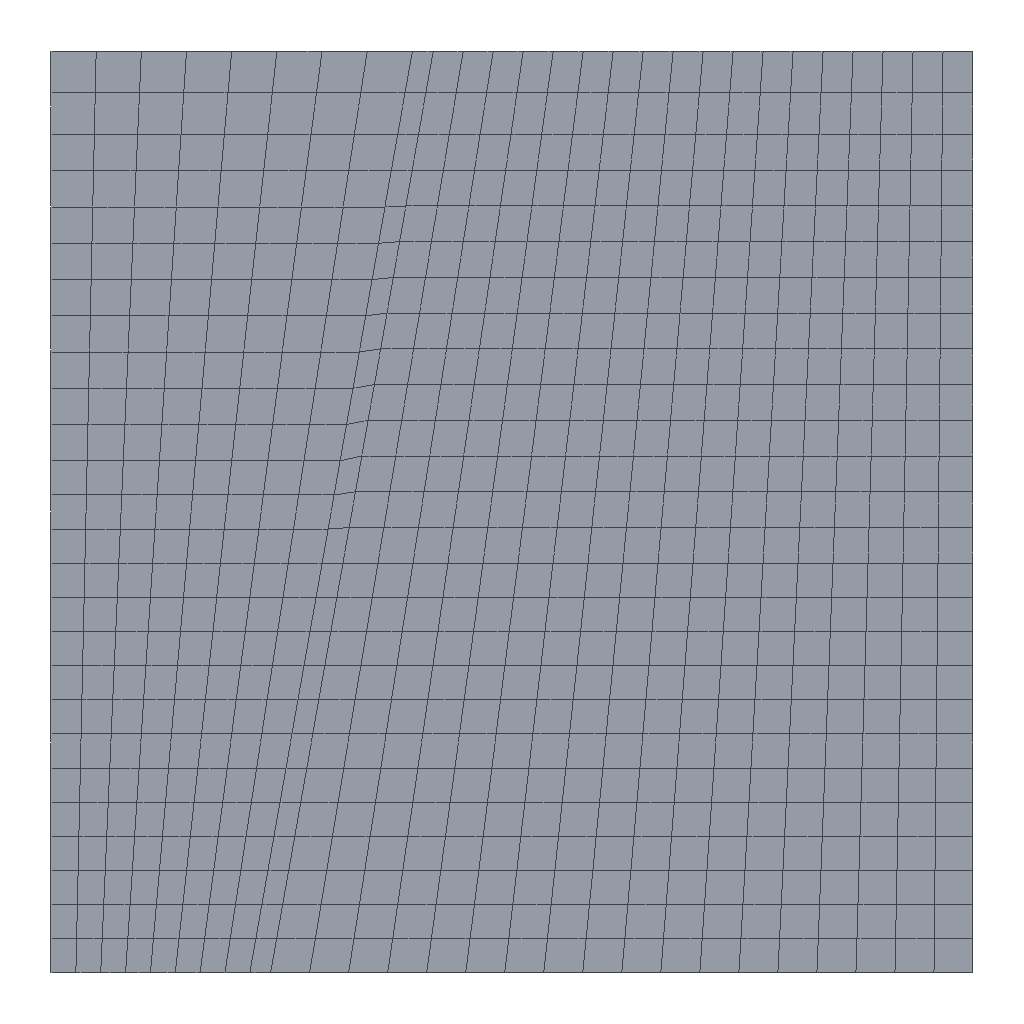Simulation study | abaqus
Set-up summary:
category,name,step,type,value,unit,region
solver,abaqus
solver,version,,,Abaqus/Standard 2020
units,not stated in the deck,,not stated
analysis,deck,,soils,soils
load_step,Step-1,Step-1,soils
load_step,requested,,,1
mesh,nodes,,,756
mesh,elements,,,702
element_type,CPE4P,,plane,702
load,load commands in deck,,count,3
bc,support commands in deck,,count,4
material,CHUSHUI,,in results
material,DUANCENG,,in results
material,DUANCENG-COPY,,in results
material,SOIL,,in results
check,setup vs results,,match,"per instance, exact: element labels, types and connectivity; labels of the nodes the elements use; coordinates of those nodes at SINGLE_PRECISION in 1 of 1 instance(s)"
Abaqus input file, long lists of numbers shortened:
*Heading
** Job name: Job-3 Model name: Model-1-Copy2
** Generated by: Abaqus/CAE 2020
*Preprint, echo=NO, model=NO, history=NO, contact=NO
**
** PARTS
**
*Part, name=Part-1
*Node
      1,           0.,  -81.506
      2,   338.411,  -81.506
** (754 more lines like these left out)
*Element, type=CPE4P
 1,   1,  21, 229,  36
 2,  21,  22, 230, 229
** (700 more lines like these left out)
*Nset, nset=Set-1
  10,  13, 118, 119
*Elset, elset=Set-1
 149, 157, 165, 529, 530, 531
*Nset, nset=Set-2
   1,   2,   3,   4,   6,   7,   9,  10,  11,  12,  13,  14,  15,  16,  21,  22
  23,  24,  25,  26,  27,  28,  29,  30,  31,  32,  33,  34,  35,  36,  38,  39
** (25 more lines like these left out)
*Elset, elset=Set-2
   1,   2,   3,   4,   5,   6,   7,   8,   9,  10,  11,  12,  13,  14,  15,  16
  53,  54,  55,  56,  57,  58,  59,  60,  61,  62,  63,  64,  65,  66,  67,  68
** (20 more lines like these left out)
*Nset, nset=Set-3
   2,   3,   5,   6,   7,   8,  28,  37,  38,  39,  40,  41,  42,  43,  44,  45
  46,  47,  48,  49,  50,  51,  52,  53,  54,  55,  56,  57,  58,  59,  60,  61
** (2 more lines like these left out)
*Elset, elset=Set-3
  17,  18,  19,  20,  21,  22,  23,  24,  25,  26,  27,  28,  29,  30,  31,  32
  33,  34,  35,  36,  37,  38,  39,  40,  41,  42,  43,  44,  45,  46,  47,  48
** (1 more lines like these left out)
*Nset, nset=Set-4
   1,   2,  13,  14,  21,  22,  23,  24,  25,  26,  27, 109, 110, 111, 112, 113
 114, 115, 120, 121, 122, 123, 124, 125, 126, 127, 128, 129, 130, 131, 132, 133
** (4 more lines like these left out)
*Elset, elset=Set-4, generate
 173,  244,    1
*Nset, nset=Set-8
   1,   2,   3,   4,   9,  10,  11,  12,  13,  14,  15,  16,  17,  18,  21,  22
  23,  24,  25,  26,  27,  28,  29,  30,  31,  32,  33,  34,  35,  36,  73,  74
** (17 more lines like these left out)
*Elset, elset=Set-8
   1,   2,   3,   4,   5,   6,   7,   8,   9,  10,  11,  12,  13,  14,  15,  16
  53,  54,  55,  56,  57,  58,  59,  60,  61,  62,  63,  64,  65,  66,  67,  68
** (13 more lines like these left out)
*Nset, nset=Set-9
   2,   3,   5,   6,   7,   8,  28,  37,  38,  39,  40,  41,  42,  43,  44,  45
  46,  47,  48,  49,  50,  51,  52,  53,  54,  55,  56,  57,  58,  59,  60,  61
** (2 more lines like these left out)
*Elset, elset=Set-9
  17,  18,  19,  20,  21,  22,  23,  24,  25,  26,  27,  28,  29,  30,  31,  32
  33,  34,  35,  36,  37,  38,  39,  40,  41,  42,  43,  44,  45,  46,  47,  48
** (1 more lines like these left out)
*Nset, nset=Set-10
   6,   7,  10,  11,  13,  14,  15,  16,  38,  39,  40,  41,  42,  43,  44,  45
  46,  47,  48,  49,  50,  51,  52,  53,  54,  84,  85,  86,  87,  88,  89,  90
** (16 more lines like these left out)
*Elset, elset=Set-10
 149, 150, 151, 152, 153, 154, 155, 156, 157, 158, 159, 160, 161, 162, 163, 164
 165, 166, 167, 168, 169, 170, 171, 172, 247, 248, 249, 250, 251, 252, 253, 254
** (13 more lines like these left out)
*Nset, nset=Set-15
   1,   2,   3,   4,   5,   6,   7,   8,   9,  10,  11,  12,  13,  14,  15,  16
  17,  18,  19,  20,  21,  22,  23,  24,  25,  26,  27,  28,  29,  30,  31,  32
** (42 more lines like these left out)
*Elset, elset=Set-15
   1,   2,   3,   4,   5,   6,   7,   8,   9,  10,  11,  12,  13,  14,  15,  16
  17,  18,  19,  20,  21,  22,  23,  24,  25,  26,  27,  28,  29,  30,  31,  32
** (36 more lines like these left out)
*Nset, nset=Set-16
  10,  11,  13,  14,  15,  16,  17,  18,  84,  85,  86,  87,  88,  89,  90, 109
 110, 111, 112, 113, 114, 115, 116, 117, 118, 119, 136, 137, 138, 139, 140, 141
** (5 more lines like these left out)
*Elset, elset=Set-16
 149, 150, 151, 152, 153, 154, 155, 156, 157, 158, 159, 160, 161, 162, 163, 164
 165, 166, 167, 168, 169, 170, 171, 172, 463, 464, 465, 466, 467, 468, 469, 470
** (3 more lines like these left out)
*Nset, nset=Set-17
   2,   3,   5,   6,   9,  10,  13,  15,  17,  19,  28,  37,  73,  74,  75,  76
  77,  78,  79,  80,  81,  82,  83, 118, 119, 128, 129, 130, 131, 132, 133, 134
** (2 more lines like these left out)
*Elset, elset=Set-17
 245, 246, 517, 518, 519, 520, 521, 522, 523, 524, 525, 526, 527, 528, 529, 530
 531, 532, 533, 534, 535, 536, 537, 538, 539, 540
*Nset, nset=Set-18
   2,   6,   9,  10,  13,  15,  17,  19,  73,  74,  75,  76,  77,  78,  79,  80
  81,  82,  83, 118, 119, 128, 129, 130, 131, 132, 133, 134, 135, 164, 165, 166
** (2 more lines like these left out)
*Elset, elset=Set-18, generate
 517,  540,    1
*Nset, nset=Set-19
  2,  3,  5,  6, 28, 37
*Elset, elset=Set-19
 245, 246
** Section: Section-soil
*Solid Section, elset=Set-15, material=soil
,
** Section: chushui
*Solid Section, elset=Set-16, material=chushui
,
** Section: ddceng
*Solid Section, elset=Set-19, material=duanceng-Copy
,
** Section: duanceng
*Solid Section, elset=Set-18, material=duanceng
,
*End Part
**
**
** ASSEMBLY
**
*Assembly, name=Assembly
**
*Instance, name=Part-1-1, part=Part-1
*End Instance
**
*Nset, nset=Set-1, instance=Part-1-1
   1,   2,   3,   4,   7,   8,  11,  13,  14,  28,  36,  55, 109, 110, 111, 112
 113, 114, 115, 116, 117
*Elset, elset=Set-1, instance=Part-1-1
   1,   8,   9,  16,  51,  52, 149, 150, 151, 152, 153, 154, 155, 156, 164, 172
 237, 238, 239, 240, 241, 242, 243, 244, 245, 246
*Nset, nset=Set-2, instance=Part-1-1
   1,   4,   7,   8,   9,  10,  11,  12,  13,  14,  16,  18,  36,  55,  84,  85
  86,  87,  88,  89,  90, 102, 103, 104, 105, 106, 107, 108, 109, 110, 111, 112
** (1 more lines like these left out)
*Elset, elset=Set-2, instance=Part-1-1
   1,   9,  51,  52,  53,  64,  65,  76,  77,  88,  89, 100, 101, 112, 113, 124
 125, 136, 137, 148, 149, 150, 151, 152, 153, 154, 155, 156, 165, 166, 167, 168
** (1 more lines like these left out)
*Nset, nset=Set-3, instance=Part-1-1
   2,   3,   5,  11,  13,  14, 116, 117, 128, 129, 130, 131, 132, 133, 134, 135
*Elset, elset=Set-3, instance=Part-1-1
 156, 164, 172, 173, 181, 189, 197, 205, 213, 221, 229, 237, 246, 532, 533, 534
 535, 536, 537, 538, 539, 540
*Nset, nset=Set-4, instance=Part-1-1
   1,   2,   3,   4,   7,   8,  11,  12,  13,  14,  28,  36,  55,  91,  92,  93
  94,  95,  96,  97,  98,  99, 100, 101, 109, 110, 111, 112, 113, 114, 115, 116
** (1 more lines like these left out)
*Elset, elset=Set-4, instance=Part-1-1
   1,   8,   9,  16,  51,  52, 137, 138, 139, 140, 141, 142, 143, 144, 145, 146
 147, 148, 149, 150, 151, 152, 153, 154, 155, 156, 164, 172, 237, 238, 239, 240
** (1 more lines like these left out)
*Nset, nset=Set-5, instance=Part-1-1
   1,   7,  14,  16, 120, 121, 122, 123, 124, 125, 126, 127, 153, 154, 155, 156
 157, 158, 159, 160, 161, 162, 163
*Elset, elset=Set-5, instance=Part-1-1
 180, 188, 196, 204, 212, 220, 228, 236, 244, 264, 282, 300, 318, 336, 354, 372
 390, 408, 426, 444, 462
*Nset, nset=Set-6, instance=Part-1-1
   9,  12,  16,  18, 102, 103, 104, 105, 106, 107, 108, 192, 193
*Elset, elset=Set-6, instance=Part-1-1
  53,  65,  77,  89, 101, 113, 125, 137, 480, 498, 516
*Nset, nset=Set-7, instance=Part-1-1
   1,   2,   3,   4,   5,   6,   7,   8,   9,  10,  11,  12,  13,  14,  15,  16
  21,  22,  23,  24,  25,  26,  27,  28,  29,  30,  31,  32,  33,  34,  35,  36
** (31 more lines like these left out)
*Elset, elset=Set-7, instance=Part-1-1, generate
   1,  462,    1
*Nset, nset=Set-8, instance=Part-1-1
   3,   4,   6,  10,  11,  12,  15,  16,  18,  29,  30,  31,  32,  33,  34,  35
  84,  85,  86,  87,  88,  89,  90,  91,  92,  93,  94,  95,  96,  97,  98,  99
** (1 more lines like these left out)
*Elset, elset=Set-8, instance=Part-1-1
   9,  10,  11,  12,  13,  14,  15,  16,  64,  76,  88, 100, 112, 124, 136, 137
 138, 139, 140, 141, 142, 143, 144, 145, 146, 147, 148, 165, 166, 167, 168, 169
** (2 more lines like these left out)
*Nset, nset=Set-9, instance=Part-1-1
   1,  14,  15,  16, 120, 121, 122, 123, 124, 125, 126, 127, 136, 137, 138, 139
 140, 141, 142, 143, 144, 145, 146, 147, 148, 149, 150, 151, 152
*Elset, elset=Set-9, instance=Part-1-1
 180, 188, 196, 204, 212, 220, 228, 236, 244, 247, 248, 249, 250, 251, 252, 253
 254, 255, 256, 257, 258, 259, 260, 261, 262, 263, 264, 499, 500, 501, 502, 503
** (1 more lines like these left out)
*Nset, nset=Set-10, instance=Part-1-1
   1,   3,   4,   5,  11,  14,  36, 116, 117
*Elset, elset=Set-10, instance=Part-1-1
   1,   9, 156, 164, 172, 246
*Nset, nset=Set-11, instance=Part-1-1
  10,  13, 118, 119
*Elset, elset=Set-11, instance=Part-1-1
 149, 157, 165, 529, 530, 531
*Nset, nset=Set-12, instance=Part-1-1
   1,   2,   3,   4,   5,   6,   7,   8,   9,  10,  11,  12,  13,  14,  15,  16
  17,  18,  19,  20,  21,  22,  23,  24,  25,  26,  27,  28,  29,  30,  31,  32
** (33 more lines like these left out)
*Elset, elset=Set-12, instance=Part-1-1
   1,   2,   3,   4,   5,   6,   7,   8,   9,  10,  11,  12,  13,  14,  15,  16
  17,  18,  19,  20,  21,  22,  23,  24,  25,  26,  27,  28,  29,  30,  31,  32
** (32 more lines like these left out)
*Nset, nset=Set-13, instance=Part-1-1
  10,  13, 118, 119
*Elset, elset=Set-13, instance=Part-1-1
 149, 157, 165, 529, 530, 531
*Nset, nset=Set-14, instance=Part-1-1
   1,   4,  11,  14,  36, 116, 117
*Elset, elset=Set-14, instance=Part-1-1
   1,   9, 156, 164, 172
*Nset, nset=Set-15, instance=Part-1-1
 3, 5
*Elset, elset=Set-15, instance=Part-1-1
 246,
*Nset, nset=Set-16, instance=Part-1-1
   1,   3,   4,   5,  11,  14,  36, 116, 117
*Elset, elset=Set-16, instance=Part-1-1
   1,   9, 156, 164, 172, 246
*Nset, nset=Set-17, instance=Part-1-1
 10, 13
*Nset, nset=Set-18, instance=Part-1-1
   1,   4,  11,  14,  36, 116, 117
*Elset, elset=Set-18, instance=Part-1-1
   1,   9, 156, 164, 172
*Nset, nset=Set-19, instance=Part-1-1
 3, 5
*Elset, elset=Set-19, instance=Part-1-1
 246,
*Nset, nset=Set-20, instance=Part-1-1
   1,   4,  11,  14,  36, 116, 117
*Elset, elset=Set-20, instance=Part-1-1
   1,   9, 156, 164, 172
*Nset, nset=Set-21, instance=Part-1-1
   5,   8,  10,  13,  56,  57,  58,  59,  60,  61,  62,  63,  64,  65,  66,  67
  68,  69,  70,  71,  72, 118, 119
*Elset, elset=Set-21, instance=Part-1-1
  17,  19,  21,  23,  25,  27,  29,  31,  33,  35,  37,  39,  41,  43,  45,  47
  49,  51, 149, 157, 165, 529, 530, 531
*Nset, nset=Set-22, instance=Part-1-1
   1,   4,  11,  14,  36, 116, 117
*Elset, elset=Set-22, instance=Part-1-1
   1,   9, 156, 164, 172, 246
*Nset, nset=Set-23, instance=Part-1-1
   1,   3,   4,   5,  11,  14,  36, 116, 117
*Elset, elset=Set-23, instance=Part-1-1
   1,   9, 156, 164, 172, 246
*Nset, nset=Set-24, instance=Part-1-1
   1,   4,  11,  14,  36, 116, 117
*Elset, elset=Set-24, instance=Part-1-1
   1,   9, 156, 164, 172
*Nset, nset=Set-25, instance=Part-1-1
   1,   4,  11,  14,  36, 116, 117
*Elset, elset=Set-25, instance=Part-1-1
   1,   9, 156, 164, 172, 246
*Nset, nset=Set-26, instance=Part-1-1
   1,   4,  11,  14,  36, 116, 117
*Elset, elset=Set-26, instance=Part-1-1
   1,   9, 156, 164, 172
*Nset, nset=Set-27, instance=Part-1-1
   1,   4,  11,  14,  36, 116, 117
*Elset, elset=Set-27, instance=Part-1-1
   1,   9, 156, 164, 172, 246
*Nset, nset=Set-28, instance=Part-1-1
   1,   4,  11,  14,  36, 116, 117
*Elset, elset=Set-28, instance=Part-1-1
   1,   9, 156, 164, 172
*Nset, nset=Set-29, instance=Part-1-1
   1,   4,  11,  14,  36, 116, 117
*Elset, elset=Set-29, instance=Part-1-1
   1,   9, 156, 164, 172, 246
*Nset, nset=Set-30, instance=Part-1-1
   2,   6,  13, 128, 129, 130, 131, 132, 133, 134, 135
*Elset, elset=Set-30, instance=Part-1-1
 173, 181, 189, 197, 205, 213, 221, 229, 237, 245, 532, 533, 534, 535, 536, 537
 538, 539, 540
*Nset, nset=Set-31, instance=Part-1-1
   2,   6,  13, 128, 129, 130, 131, 132, 133, 134, 135
*Elset, elset=Set-31, instance=Part-1-1
 173, 181, 189, 197, 205, 213, 221, 229, 237, 245, 532, 533, 534, 535, 536, 537
 538, 539, 540
*Nset, nset=Set-32, instance=Part-1-1
   2,   3,   4,  11,  12,  13,  14,  29,  30,  31,  32,  33,  34,  35,  91,  92
  93,  94,  95,  96,  97,  98,  99, 100, 101, 109, 110, 111, 112, 113, 114, 115
** (1 more lines like these left out)
*Elset, elset=Set-32, instance=Part-1-1
   9,  10,  11,  12,  13,  14,  15,  16, 137, 138, 139, 140, 141, 142, 143, 144
 145, 146, 147, 148, 149, 150, 151, 152, 153, 154, 155, 156, 173, 181, 189, 197
** (2 more lines like these left out)
*Nset, nset=Set-33, instance=Part-1-1
   1,   2,   4,   6,  15,  17,  36, 194, 195
*Elset, elset=Set-33, instance=Part-1-1
   1,   9, 245, 463, 481, 499, 526, 527, 528, 540
*Nset, nset=Set-34, instance=Part-1-1
   7,  10,  13,  16, 118, 119, 153, 154, 155, 156, 157, 158, 159, 160, 161, 162
 163,
*Elset, elset=Set-34, instance=Part-1-1
 149, 157, 165, 264, 282, 300, 318, 336, 354, 372, 390, 408, 426, 444, 462, 529
 530, 531
*Nset, nset=Set-35, instance=Part-1-1
   1,   2,   3,   4,   5,   6,   7,   8,   9,  10,  11,  12,  13,  14,  15,  16
  17,  18,  21,  22,  23,  24,  25,  26,  27,  28,  29,  30,  31,  32,  33,  34
** (35 more lines like these left out)
*Elset, elset=Set-35, instance=Part-1-1, generate
   1,  516,    1
*Nset, nset=Set-36, instance=Part-1-1
   2,  10,  11,  13,  84,  85,  86,  87,  88,  89,  90, 128, 129, 130, 131, 132
 133, 134, 135
*Elset, elset=Set-36, instance=Part-1-1
  64,  76,  88, 100, 112, 124, 136, 148, 165, 166, 167, 168, 169, 170, 171, 172
 173, 181, 189, 197, 205, 213, 221, 229, 237, 532, 533, 534, 535, 536, 537, 538
** (1 more lines like these left out)
*Nset, nset=Set-38, instance=Part-1-1
   2,   6,  13, 128, 129, 130, 131, 132, 133, 134, 135
*Elset, elset=Set-38, instance=Part-1-1
 173, 181, 189, 197, 205, 213, 221, 229, 237, 245, 532, 533, 534, 535, 536, 537
 538, 539, 540
*Nset, nset=Set-39, instance=Part-1-1
   1,   4,   7,   8,  11,  12,  14,  16,  18,  20,  36,  55,  91,  92,  93,  94
  95,  96,  97,  98,  99, 100, 101, 116, 117, 120, 121, 122, 123, 124, 125, 126
** (2 more lines like these left out)
*Elset, elset=Set-39, instance=Part-1-1
   1,   9,  51,  52, 137, 138, 139, 140, 141, 142, 143, 144, 145, 146, 147, 148
 156, 164, 172, 180, 188, 196, 204, 212, 220, 228, 236, 244, 264, 282, 300, 318
** (2 more lines like these left out)
*Nset, nset=Set-40, instance=Part-1-1
   9,  12,  19,  20, 102, 103, 104, 105, 106, 107, 108, 204, 205, 206, 207, 208
 209, 210, 211, 212, 213, 214, 215, 216, 217, 218, 219, 220
*Elset, elset=Set-40, instance=Part-1-1
  53,  65,  77,  89, 101, 113, 125, 137, 517, 549, 558, 567, 576, 585, 594, 603
 612, 621, 630, 639, 648, 657, 666, 675, 684, 693, 702
*Nset, nset=Set-41, instance=Part-1-1
  10,  13,  15,  17, 118, 119, 194, 195
*Elset, elset=Set-41, instance=Part-1-1
 149, 157, 165, 463, 481, 499, 526, 527, 528, 529, 530, 531
*Nset, nset=Set-42, instance=Part-1-1
  1,  7, 21, 22, 23, 24, 25, 26, 27, 38, 39, 40, 41, 42, 43, 44
 45, 46, 47, 48, 49, 50, 51, 52, 53, 54
*Elset, elset=Set-42, instance=Part-1-1
   1,   2,   3,   4,   5,   6,   7,   8,  18,  20,  22,  24,  26,  28,  30,  32
  34,  36,  38,  40,  42,  44,  46,  48,  50,  52, 173, 174, 175, 176, 177, 178
** (2 more lines like these left out)
*Nset, nset=Set-43, instance=Part-1-1, generate
   1,  756,    1
*Elset, elset=Set-43, instance=Part-1-1, generate
   1,  702,    1
*Nset, nset=Set-44, instance=Part-1-1, generate
   1,  756,    1
*Elset, elset=Set-44, instance=Part-1-1, generate
   1,  702,    1
*Nset, nset=Set-45, instance=Part-1-1
  3,  4,  5,  8, 29, 30, 31, 32, 33, 34, 35, 56, 57, 58, 59, 60
 61, 62, 63, 64, 65, 66, 67, 68, 69, 70, 71, 72
*Elset, elset=Set-45, instance=Part-1-1
   9,  10,  11,  12,  13,  14,  15,  16,  17,  19,  21,  23,  25,  27,  29,  31
  33,  35,  37,  39,  41,  43,  45,  47,  49,  51, 246
*Nset, nset=Set-46, instance=Part-1-1
 3, 5
*Nset, nset=Set-47, instance=Part-1-1
 3, 5
*Elset, elset=Set-47, instance=Part-1-1
 246,
*Nset, nset=Set-48, instance=Part-1-1
  10,  13, 118, 119
*Elset, elset=Set-48, instance=Part-1-1
 149, 157, 165, 529, 530, 531
*Elset, elset=_Surf-1_S4, internal, instance=Part-1-1, generate
  53,  137,   12
*Elset, elset=_Surf-1_S2, internal, instance=Part-1-1, generate
 480,  516,   18
*Surface, type=ELEMENT, name=Surf-1
_Surf-1_S4, S4
_Surf-1_S2, S2
*Elset, elset=_Surf-2_S4, internal, instance=Part-1-1
 1, 9
*Elset, elset=_Surf-2_S2, internal, instance=Part-1-1
 156, 164, 172, 246
*Surface, type=ELEMENT, name=Surf-2
_Surf-2_S4, S4
_Surf-2_S2, S2
*Elset, elset=_Surf-3_S4, internal, instance=Part-1-1
 1, 9
*Elset, elset=_Surf-3_S2, internal, instance=Part-1-1, generate
 156,  172,    8
*Surface, type=ELEMENT, name=Surf-3
_Surf-3_S4, S4
_Surf-3_S2, S2
*Elset, elset=_Surf-4_S4, internal, instance=Part-1-1
 1, 9
*Elset, elset=_Surf-4_S2, internal, instance=Part-1-1
 156, 164, 172, 246
*Surface, type=ELEMENT, name=Surf-4
_Surf-4_S4, S4
_Surf-4_S2, S2
*Elset, elset=_Surf-5_S4, internal, instance=Part-1-1
 1, 9
*Elset, elset=_Surf-5_S2, internal, instance=Part-1-1, generate
 156,  172,    8
*Surface, type=ELEMENT, name=Surf-5
_Surf-5_S4, S4
_Surf-5_S2, S2
*Elset, elset=_Surf-6_S4, internal, instance=Part-1-1
 1, 9
*Elset, elset=_Surf-6_S2, internal, instance=Part-1-1
 156, 164, 172, 246
*Surface, type=ELEMENT, name=Surf-6
_Surf-6_S4, S4
_Surf-6_S2, S2
*Elset, elset=_Surf-7_S4, internal, instance=Part-1-1
 1, 9
*Elset, elset=_Surf-7_S2, internal, instance=Part-1-1, generate
 156,  172,    8
*Surface, type=ELEMENT, name=Surf-7
_Surf-7_S4, S4
_Surf-7_S2, S2
*Elset, elset=_Surf-8_S4, internal, instance=Part-1-1
 1, 9
*Elset, elset=_Surf-8_S2, internal, instance=Part-1-1
 156, 164, 172, 246
*Surface, type=ELEMENT, name=Surf-8
_Surf-8_S4, S4
_Surf-8_S2, S2
*Elset, elset=_Surf-9_S4, internal, instance=Part-1-1
 245,
*Elset, elset=_Surf-9_S3, internal, instance=Part-1-1, generate
 532,  540,    1
*Surface, type=ELEMENT, name=Surf-9
_Surf-9_S4, S4
_Surf-9_S3, S3
*Elset, elset=_Surf-10_S3, internal, instance=Part-1-1
 165, 166, 167, 168, 169, 170, 171, 172, 532, 533, 534, 535, 536, 537, 538, 539
 540,
*Surface, type=ELEMENT, name=Surf-10
_Surf-10_S3, S3
*Elset, elset=_Surf-11_S3, internal, instance=Part-1-1, generate
 532,  540,    1
*Surface, type=ELEMENT, name=Surf-11
_Surf-11_S3, S3
*Elset, elset=_Surf-12_S3, internal, instance=Part-1-1, generate
  9,  16,   1
*Elset, elset=_Surf-12_S4, internal, instance=Part-1-1, generate
 17,  51,   2
*Elset, elset=_Surf-12_S2, internal, instance=Part-1-1
 246,
*Surface, type=ELEMENT, name=Surf-12
_Surf-12_S3, S3
_Surf-12_S4, S4
_Surf-12_S2, S2
*Elset, elset=_Surf-13_S3, internal, instance=Part-1-1, generate
  9,  16,   1
*Elset, elset=_Surf-13_S4, internal, instance=Part-1-1, generate
 17,  51,   2
*Surface, type=ELEMENT, name=Surf-13
_Surf-13_S3, S3
_Surf-13_S4, S4
*Nset, nset=Set-48_PP_, internal, instance=Part-1-1
  10,  13, 118, 119
*Nset, nset=Set-42_PP_, internal, instance=Part-1-1
  1,  7, 21, 22, 23, 24, 25, 26, 27, 38, 39, 40, 41, 42, 43, 44
 45, 46, 47, 48, 49, 50, 51, 52, 53, 54
*End Assembly
*Amplitude, name=Amp-1
             0.,              0.,              1.,              1.
**
** MATERIALS
**
*Material, name=chushui
*Density
2200.,
*Elastic
 1.44e+10, 0.2
*Gap Flow
 0.001,
*Permeability, specific=9980.
 1.5e-13, 0.19
*Material, name=duanceng
*Density
2200.,
*Elastic
 1.44e+10, 0.2
*Gap Flow
 0.001,
*Permeability, specific=9980.
 1.5e-09, 0.19
*Material, name=duanceng-Copy
*Density
2200.,
*Elastic
 1.44e+10, 0.2
*Gap Flow
 0.001,
*Permeability, specific=9980.
0., 0.0001
*Material, name=soil
*Density
2500.,
*Elastic
 2.964e+10, 0.12
*Gap Flow
 0.001,
*Permeability, specific=9980.
 2e-16, 0.04
**
** BOUNDARY CONDITIONS
**
** Name: BC-1 Type: 位移/转角
*Boundary
Set-39, 1, 1
** Name: BC-2 Type: 位移/转角
*Boundary
Set-40, 2, 2
**
** PREDEFINED FIELDS
**
** Name: Predefined Field-1   Type: Stress
*Initial Conditions, type=STRESS
Set-43, 0., 0., 0., 0.,
** Name: Predefined Field-2   Type: Void ratio
*Initial Conditions, TYPE=RATIO
Set-44, 1.
** ----------------------------------------------------------------
**
** STEP: Step-1
**
*Step, name=Step-1, nlgeom=YES, inc=1000
*Soils, utol=1.0, creep=none, stabilize=0.0002, allsdtol=0.05, continue=NO
0.01, 1., 1e-05, 1.,
**
** BOUNDARY CONDITIONS
**
** Name: BC-4 Type: 孔隙压力
*Boundary
Set-48_PP_, 8, 8, 1e+08
** Name: [REDACTED] : Pore pressure
*Boundary
Set-42_PP_, 8, 8, 3e+06
**
** LOADS
**
** Name: Load-pressure   Type: Pressure
*Dsload
Surf-13, P, 7.36e+06
**
** OUTPUT REQUESTS
**
*Restart, write, frequency=0
**
** FIELD OUTPUT: F-Output-1
**
*Output, field
*Node Output
CF, POR, RF, U, V
*Element Output, directions=YES
E, FLUVR, FLVEL, LE, MISES, MISESMAX, PE, S, SAT, VOIDR, PEEQ
*Contact Output
PFL, PFLA, PTL, PTLA
**
** HISTORY OUTPUT: H-Output-1
**
*Output, history, variable=PRESELECT
*End Step
Results summary:
result,step,,completed,increments=11 time=1.0/1.0
result,analysis,,,soils
result,last_loadstep,,,1
result,primary field,,,"U, POR"
result,reaction total,,FX,1547392.0,model units
result,reaction total,,FY,6474085352.5,model units
result,reaction total,,FZ,0.0,model units